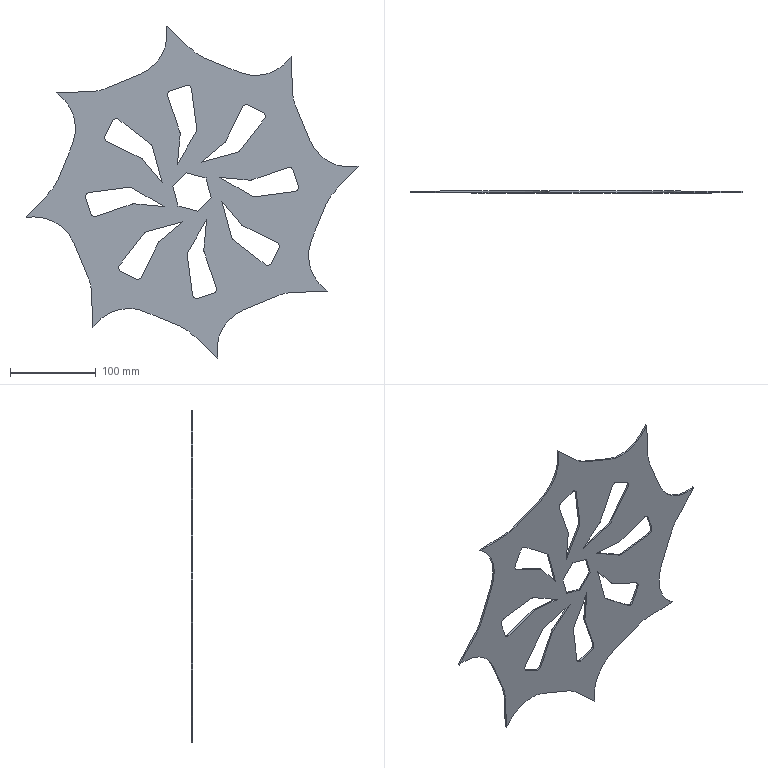Part | SolidWorks | features ICE 3, Extrusion 1, Fillet 1 | 1 solid | 128 faces | box 387.128 x 2 x 387.128 mm | volume 134458 mm3 | plane 72 | cylinder 56 | commonest cylinder face diameters 10 x38 100 x18